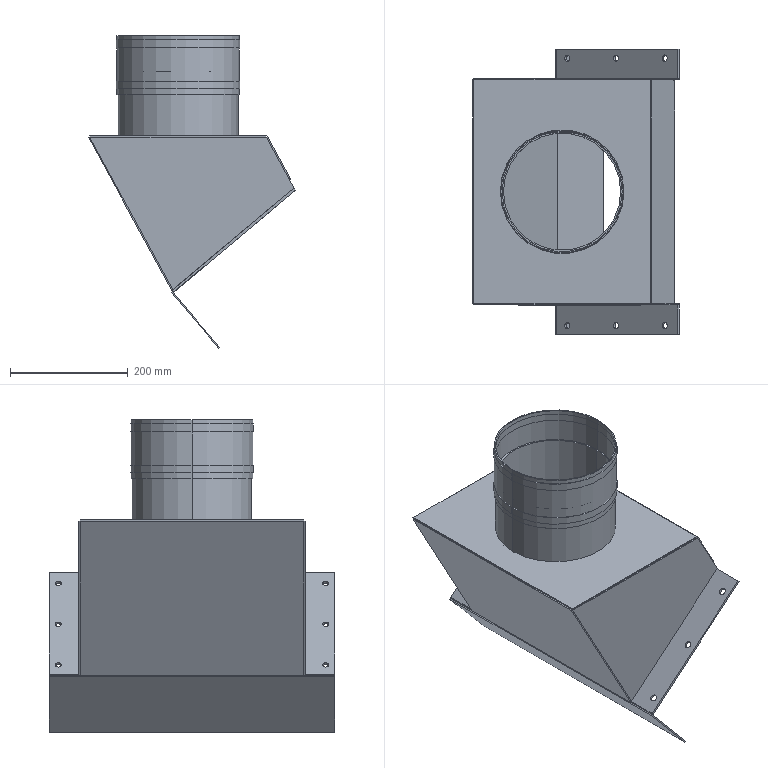Part | STEP file | EXHAUST1V11 | 12 solids | 88 faces | box 350.686 x 484 x 530.45 mm | volume 1247734 mm3 | plane 56 | cylinder 32 | commonest cylinder face diameters 11 x12 204 x8 199 x4 210 x4 10 x2 208 x2